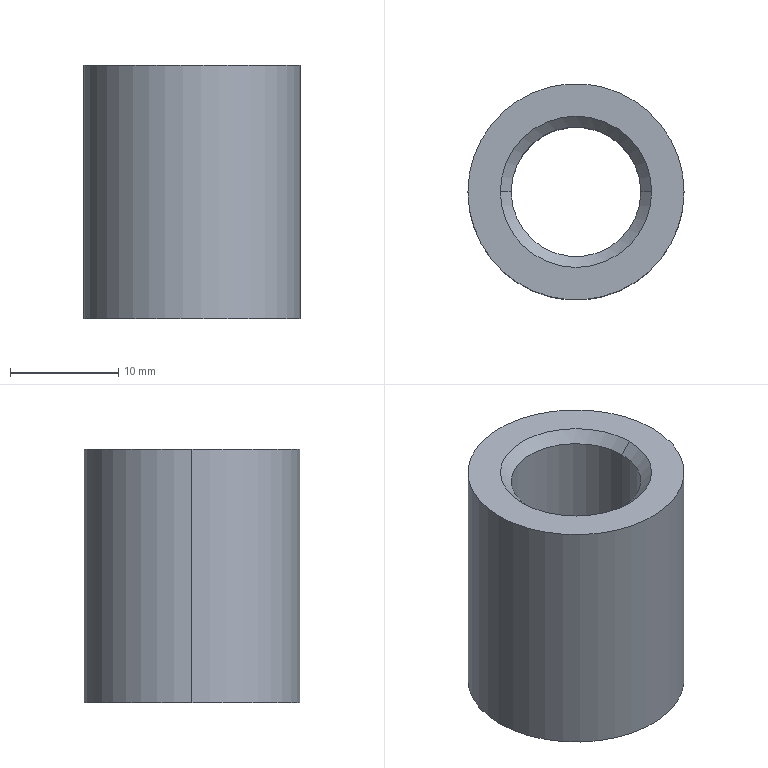Part | STEP file | 塑料轴套内10外20长20 Copy | 1 solid | 10 faces | box 20 x 20 x 23.5 mm | volume 4685 mm3 | cone 4 | cylinder 4 | plane 2 | commonest cylinder face diameters 12 x2 20 x2
STEP:
#1=CARTESIAN_POINT('',(6.,0.,1.));
#2=VERTEX_POINT('',#1);
#3=CARTESIAN_POINT('',(-6.,0.,1.));
#4=VERTEX_POINT('',#3);
#5=CARTESIAN_POINT('',(0.,0.,1.));
#6=DIRECTION('',(0.,0.,-1.));
#7=DIRECTION('',(1.,0.,0.));
#8=AXIS2_PLACEMENT_3D('',#5,#6,#7);
#9=CIRCLE('',#8,6.);
#10=EDGE_CURVE('',#2,#4,#9,.T.);
#11=ORIENTED_EDGE('',*,*,#10,.F.);
#12=CARTESIAN_POINT('',(7.,0.,0.));
#13=VERTEX_POINT('',#12);
#14=CARTESIAN_POINT('',(7.,0.,0.));
#15=DIRECTION('',(0.7071,0.,-0.7071));
#16=VECTOR('',#15,1000.);
#17=LINE('',#14,#16);
#18=EDGE_CURVE('',#2,#13,#17,.T.);
#19=ORIENTED_EDGE('',*,*,#18,.T.);
#20=CARTESIAN_POINT('',(-7.,0.,0.));
#21=VERTEX_POINT('',#20);
#22=CARTESIAN_POINT('',(0.,0.,0.));
#23=DIRECTION('',(0.,0.,1.));
#24=DIRECTION('',(1.,0.,0.));
#25=AXIS2_PLACEMENT_3D('',#22,#23,#24);
#26=CIRCLE('',#25,7.);
#27=EDGE_CURVE('',#21,#13,#26,.T.);
#28=ORIENTED_EDGE('',*,*,#27,.F.);
#29=CARTESIAN_POINT('',(-7.,0.,0.));
#30=DIRECTION('',(-0.7071,0.,-0.7071));
#31=VECTOR('',#30,1000.);
#32=LINE('',#29,#31);
#33=EDGE_CURVE('',#4,#21,#32,.T.);
#34=ORIENTED_EDGE('',*,*,#33,.F.);
#35=EDGE_LOOP('',(#11,#19,#28,#34));
#36=FACE_OUTER_BOUND('',#35,.T.);
#37=CARTESIAN_POINT('',(0.,0.,0.));
#38=DIRECTION('',(0.,0.,-1.));
#39=DIRECTION('',(-1.,0.,0.));
#40=AXIS2_PLACEMENT_3D('',#37,#38,#39);
#41=CONICAL_SURFACE('',#40,7.,0.7854);
#42=ADVANCED_FACE('',(#36),#41,.F.);
#43=CARTESIAN_POINT('',(-6.,0.,22.5));
#44=VERTEX_POINT('',#43);
#45=CARTESIAN_POINT('',(6.,0.,22.5));
#46=VERTEX_POINT('',#45);
#47=CARTESIAN_POINT('',(0.,0.,22.5));
#48=DIRECTION('',(0.,0.,1.));
#49=DIRECTION('',(1.,0.,0.));
#50=AXIS2_PLACEMENT_3D('',#47,#48,#49);
#51=CIRCLE('',#50,6.);
#52=EDGE_CURVE('',#44,#46,#51,.T.);
#53=ORIENTED_EDGE('',*,*,#52,.F.);
#54=CARTESIAN_POINT('',(-7.,0.,23.5));
#55=VERTEX_POINT('',#54);
#56=CARTESIAN_POINT('',(-6.,0.,22.5));
#57=DIRECTION('',(-0.7071,0.,0.7071));
#58=VECTOR('',#57,1000.);
#59=LINE('',#56,#58);
#60=EDGE_CURVE('',#44,#55,#59,.T.);
#61=ORIENTED_EDGE('',*,*,#60,.T.);
#62=CARTESIAN_POINT('',(7.,0.,23.5));
#63=VERTEX_POINT('',#62);
#64=CARTESIAN_POINT('',(0.,0.,23.5));
#65=DIRECTION('',(0.,0.,-1.));
#66=DIRECTION('',(1.,0.,0.));
#67=AXIS2_PLACEMENT_3D('',#64,#65,#66);
#68=CIRCLE('',#67,7.);
#69=EDGE_CURVE('',#63,#55,#68,.T.);
#70=ORIENTED_EDGE('',*,*,#69,.F.);
#71=CARTESIAN_POINT('',(6.,0.,22.5));
#72=DIRECTION('',(0.7071,0.,0.7071));
#73=VECTOR('',#72,1000.);
#74=LINE('',#71,#73);
#75=EDGE_CURVE('',#46,#63,#74,.T.);
#76=ORIENTED_EDGE('',*,*,#75,.F.);
#77=EDGE_LOOP('',(#53,#61,#70,#76));
#78=FACE_OUTER_BOUND('',#77,.T.);
#79=CARTESIAN_POINT('',(0.,0.,22.5));
#80=DIRECTION('',(0.,0.,1.));
#81=DIRECTION('',(1.,0.,0.));
#82=AXIS2_PLACEMENT_3D('',#79,#80,#81);
#83=CONICAL_SURFACE('',#82,6.,0.7854);
#84=ADVANCED_FACE('',(#78),#83,.F.);
#85=ORIENTED_EDGE('',*,*,#52,.T.);
#86=CARTESIAN_POINT('',(6.,0.,23.5));
#87=DIRECTION('',(0.,0.,-1.));
#88=VECTOR('',#87,1000.);
#89=LINE('',#86,#88);
#90=EDGE_CURVE('',#46,#2,#89,.T.);
#91=ORIENTED_EDGE('',*,*,#90,.T.);
#92=ORIENTED_EDGE('',*,*,#10,.T.);
#93=CARTESIAN_POINT('',(-6.,0.,23.5));
#94=DIRECTION('',(0.,0.,-1.));
#95=VECTOR('',#94,1000.);
#96=LINE('',#93,#95);
#97=EDGE_CURVE('',#44,#4,#96,.T.);
#98=ORIENTED_EDGE('',*,*,#97,.F.);
#99=EDGE_LOOP('',(#85,#91,#92,#98));
#100=FACE_OUTER_BOUND('',#99,.T.);
#101=CARTESIAN_POINT('',(0.,0.,23.5));
#102=DIRECTION('',(0.,0.,-1.));
#103=DIRECTION('',(-1.,0.,0.));
#104=AXIS2_PLACEMENT_3D('',#101,#102,#103);
#105=CYLINDRICAL_SURFACE('',#104,6.);
#106=ADVANCED_FACE('',(#100),#105,.F.);
#107=CARTESIAN_POINT('',(10.,0.,23.5));
#108=VERTEX_POINT('',#107);
#109=CARTESIAN_POINT('',(-10.,0.,23.5));
#110=VERTEX_POINT('',#109);
#111=CARTESIAN_POINT('',(0.,0.,23.5));
#112=DIRECTION('',(0.,0.,1.));
#113=DIRECTION('',(1.,0.,0.));
#114=AXIS2_PLACEMENT_3D('',#111,#112,#113);
#115=CIRCLE('',#114,10.);
#116=EDGE_CURVE('',#108,#110,#115,.T.);
#117=ORIENTED_EDGE('',*,*,#116,.F.);
#118=CARTESIAN_POINT('',(10.,0.,0.));
#119=VERTEX_POINT('',#118);
#120=CARTESIAN_POINT('',(10.,0.,23.5));
#121=DIRECTION('',(0.,0.,-1.));
#122=VECTOR('',#121,1000.);
#123=LINE('',#120,#122);
#124=EDGE_CURVE('',#108,#119,#123,.T.);
#125=ORIENTED_EDGE('',*,*,#124,.T.);
#126=CARTESIAN_POINT('',(-10.,0.,0.));
#127=VERTEX_POINT('',#126);
#128=CARTESIAN_POINT('',(0.,0.,0.));
#129=DIRECTION('',(0.,0.,1.));
#130=DIRECTION('',(1.,0.,0.));
#131=AXIS2_PLACEMENT_3D('',#128,#129,#130);
#132=CIRCLE('',#131,10.);
#133=EDGE_CURVE('',#119,#127,#132,.T.);
#134=ORIENTED_EDGE('',*,*,#133,.T.);
#135=CARTESIAN_POINT('',(-10.,0.,23.5));
#136=DIRECTION('',(0.,0.,-1.));
#137=VECTOR('',#136,1000.);
#138=LINE('',#135,#137);
#139=EDGE_CURVE('',#110,#127,#138,.T.);
#140=ORIENTED_EDGE('',*,*,#139,.F.);
#141=EDGE_LOOP('',(#117,#125,#134,#140));
#142=FACE_OUTER_BOUND('',#141,.T.);
#143=CARTESIAN_POINT('',(0.,0.,23.5));
#144=DIRECTION('',(0.,0.,-1.));
#145=DIRECTION('',(-1.,0.,0.));
#146=AXIS2_PLACEMENT_3D('',#143,#144,#145);
#147=CYLINDRICAL_SURFACE('',#146,10.);
#148=ADVANCED_FACE('',(#142),#147,.T.);
#149=ORIENTED_EDGE('',*,*,#69,.T.);
#150=CARTESIAN_POINT('',(0.,0.,23.5));
#151=DIRECTION('',(0.,0.,-1.));
#152=DIRECTION('',(1.,0.,0.));
#153=AXIS2_PLACEMENT_3D('',#150,#151,#152);
#154=CIRCLE('',#153,7.);
#155=EDGE_CURVE('',#55,#63,#154,.T.);
#156=ORIENTED_EDGE('',*,*,#155,.T.);
#157=EDGE_LOOP('',(#149,#156));
#158=FACE_BOUND('',#157,.T.);
#159=CARTESIAN_POINT('',(0.,0.,23.5));
#160=DIRECTION('',(0.,0.,1.));
#161=DIRECTION('',(1.,0.,0.));
#162=AXIS2_PLACEMENT_3D('',#159,#160,#161);
#163=CIRCLE('',#162,10.);
#164=EDGE_CURVE('',#110,#108,#163,.T.);
#165=ORIENTED_EDGE('',*,*,#164,.T.);
#166=ORIENTED_EDGE('',*,*,#116,.T.);
#167=EDGE_LOOP('',(#165,#166));
#168=FACE_OUTER_BOUND('',#167,.T.);
#169=CARTESIAN_POINT('',(0.,0.,23.5));
#170=DIRECTION('',(0.,0.,1.));
#171=DIRECTION('',(1.,0.,0.));
#172=AXIS2_PLACEMENT_3D('',#169,#170,#171);
#173=PLANE('',#172);
#174=ADVANCED_FACE('',(#158,#168),#173,.T.);
#175=ORIENTED_EDGE('',*,*,#27,.T.);
#176=CARTESIAN_POINT('',(0.,0.,0.));
#177=DIRECTION('',(0.,0.,1.));
#178=DIRECTION('',(1.,0.,0.));
#179=AXIS2_PLACEMENT_3D('',#176,#177,#178);
#180=CIRCLE('',#179,7.);
#181=EDGE_CURVE('',#13,#21,#180,.T.);
#182=ORIENTED_EDGE('',*,*,#181,.T.);
#183=EDGE_LOOP('',(#175,#182));
#184=FACE_BOUND('',#183,.T.);
#185=CARTESIAN_POINT('',(0.,0.,0.));
#186=DIRECTION('',(0.,0.,1.));
#187=DIRECTION('',(1.,0.,0.));
#188=AXIS2_PLACEMENT_3D('',#185,#186,#187);
#189=CIRCLE('',#188,10.);
#190=EDGE_CURVE('',#127,#119,#189,.T.);
#191=ORIENTED_EDGE('',*,*,#190,.F.);
#192=ORIENTED_EDGE('',*,*,#133,.F.);
#193=EDGE_LOOP('',(#191,#192));
#194=FACE_OUTER_BOUND('',#193,.T.);
#195=CARTESIAN_POINT('',(0.,0.,0.));
#196=DIRECTION('',(0.,0.,1.));
#197=DIRECTION('',(1.,0.,0.));
#198=AXIS2_PLACEMENT_3D('',#195,#196,#197);
#199=PLANE('',#198);
#200=ADVANCED_FACE('',(#184,#194),#199,.F.);
#201=ORIENTED_EDGE('',*,*,#124,.F.);
#202=ORIENTED_EDGE('',*,*,#164,.F.);
#203=ORIENTED_EDGE('',*,*,#139,.T.);
#204=ORIENTED_EDGE('',*,*,#190,.T.);
#205=EDGE_LOOP('',(#201,#202,#203,#204));
#206=FACE_OUTER_BOUND('',#205,.T.);
#207=CARTESIAN_POINT('',(0.,0.,23.5));
#208=DIRECTION('',(0.,0.,-1.));
#209=DIRECTION('',(-1.,0.,0.));
#210=AXIS2_PLACEMENT_3D('',#207,#208,#209);
#211=CYLINDRICAL_SURFACE('',#210,10.);
#212=ADVANCED_FACE('',(#206),#211,.T.);
#213=ORIENTED_EDGE('',*,*,#90,.F.);
#214=CARTESIAN_POINT('',(0.,0.,22.5));
#215=DIRECTION('',(0.,0.,1.));
#216=DIRECTION('',(1.,0.,0.));
#217=AXIS2_PLACEMENT_3D('',#214,#215,#216);
#218=CIRCLE('',#217,6.);
#219=EDGE_CURVE('',#46,#44,#218,.T.);
#220=ORIENTED_EDGE('',*,*,#219,.T.);
#221=ORIENTED_EDGE('',*,*,#97,.T.);
#222=CARTESIAN_POINT('',(0.,0.,1.));
#223=DIRECTION('',(0.,0.,-1.));
#224=DIRECTION('',(1.,0.,0.));
#225=AXIS2_PLACEMENT_3D('',#222,#223,#224);
#226=CIRCLE('',#225,6.);
#227=EDGE_CURVE('',#4,#2,#226,.T.);
#228=ORIENTED_EDGE('',*,*,#227,.T.);
#229=EDGE_LOOP('',(#213,#220,#221,#228));
#230=FACE_OUTER_BOUND('',#229,.T.);
#231=CARTESIAN_POINT('',(0.,0.,23.5));
#232=DIRECTION('',(0.,0.,-1.));
#233=DIRECTION('',(-1.,0.,0.));
#234=AXIS2_PLACEMENT_3D('',#231,#232,#233);
#235=CYLINDRICAL_SURFACE('',#234,6.);
#236=ADVANCED_FACE('',(#230),#235,.F.);
#237=ORIENTED_EDGE('',*,*,#60,.F.);
#238=ORIENTED_EDGE('',*,*,#219,.F.);
#239=ORIENTED_EDGE('',*,*,#75,.T.);
#240=ORIENTED_EDGE('',*,*,#155,.F.);
#241=EDGE_LOOP('',(#237,#238,#239,#240));
#242=FACE_OUTER_BOUND('',#241,.T.);
#243=CARTESIAN_POINT('',(0.,0.,22.5));
#244=DIRECTION('',(0.,0.,1.));
#245=DIRECTION('',(1.,0.,0.));
#246=AXIS2_PLACEMENT_3D('',#243,#244,#245);
#247=CONICAL_SURFACE('',#246,6.,0.7854);
#248=ADVANCED_FACE('',(#242),#247,.F.);
#249=ORIENTED_EDGE('',*,*,#18,.F.);
#250=ORIENTED_EDGE('',*,*,#227,.F.);
#251=ORIENTED_EDGE('',*,*,#33,.T.);
#252=ORIENTED_EDGE('',*,*,#181,.F.);
#253=EDGE_LOOP('',(#249,#250,#251,#252));
#254=FACE_OUTER_BOUND('',#253,.T.);
#255=CARTESIAN_POINT('',(0.,0.,0.));
#256=DIRECTION('',(0.,0.,-1.));
#257=DIRECTION('',(-1.,0.,0.));
#258=AXIS2_PLACEMENT_3D('',#255,#256,#257);
#259=CONICAL_SURFACE('',#258,7.,0.7854);
#260=ADVANCED_FACE('',(#254),#259,.F.);
#261=CLOSED_SHELL('',(#42,#84,#106,#148,#174,#200,#212,#236,#248,#260));
#262=MANIFOLD_SOLID_BREP('',#261);
#263=CARTESIAN_POINT('',(0.,0.,0.));
#264=DIRECTION('',(0.,0.,1.));
#265=DIRECTION('',(1.,0.,0.));
#266=AXIS2_PLACEMENT_3D('',#263,#264,#265);
#267=(LENGTH_UNIT()NAMED_UNIT(*)SI_UNIT(.MILLI.,.METRE.));
#268=UNCERTAINTY_MEASURE_WITH_UNIT(LENGTH_MEASURE(0.00001),#267,'','');
#269=(NAMED_UNIT(*)PLANE_ANGLE_UNIT()SI_UNIT($,.RADIAN.));
#270=(NAMED_UNIT(*)SI_UNIT($,.STERADIAN.)SOLID_ANGLE_UNIT());
#271=(GEOMETRIC_REPRESENTATION_CONTEXT(3)GLOBAL_UNCERTAINTY_ASSIGNED_CONTEXT((#268))GLOBAL_UNIT_ASSIGNED_CONTEXT((#267,#269,#270))REPRESENTATION_CONTEXT('',''));
#272=ADVANCED_BREP_SHAPE_REPRESENTATION('',(#262,#266),#271);